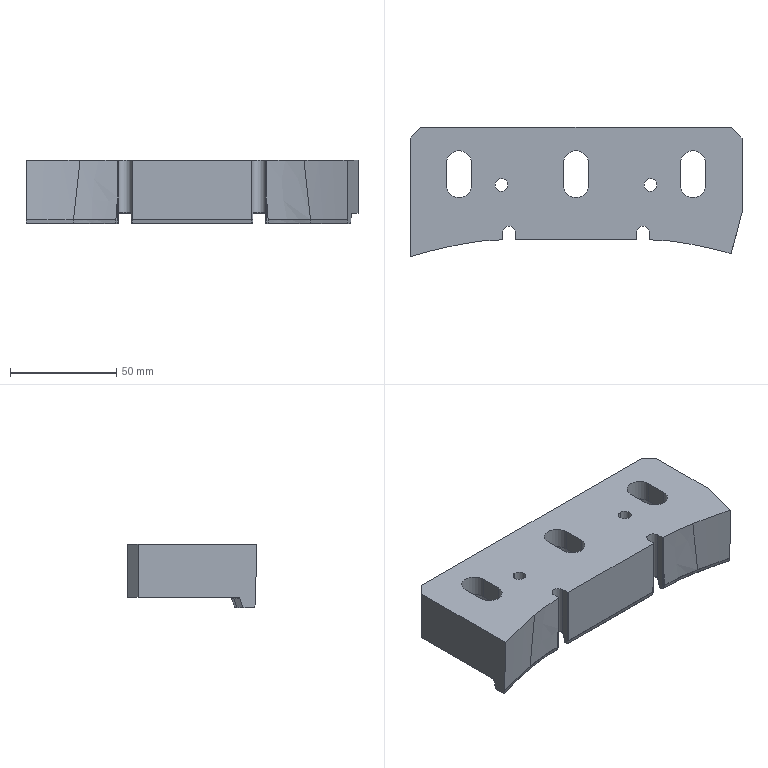CAM job | Mastercam | 3-axis milling | part box 156 x 60.706 x 30 mm
Tools:
tool_number,name,type,diameter_mm,corner_radius_mm,flutes,flute_length_mm,overall_length_mm,shoulder_length_mm,holder_diameter_mm,length_offset,diameter_offset,default_rpm,default_feed_mm_min,default_plunge_mm_min,coolant
1,63 Flat End Mill,end mill,63,0,4,25,75,25,50,1,1,159,19.08,600,COOL_OFF
2,6 Flat End Mill,end mill,6,0,4,25,75,25,50,2,2,1667,200.04,600,COOL_OFF
4,4 Flat End Mill,end mill,4,0,4,25,75,25,50,4,4,2500,300,600,COOL_OFF
6,6 Flat End Mill,end mill,6,0,4,25,75,25,50,6,6,1667,200.04,600,COOL_OFF
10,10 Flat End Mill,end mill,10,0,4,25,75,25,50,10,10,1000,120,600,COOL_OFF
11,10 Flat End Mill,end mill,10,0,4,25,75,25,50,11,11,1000,120,600,COOL_OFF
14,4 Flat End Mill,end mill,4,0,4,25,75,25,50,14,14,2500,300,600,COOL_OFF
16,16 Flat End Mill,end mill,16,0,4,25,100,25,50,16,16,750,90,600,COOL_OFF
17,12 Bull Nose Mill,bull end mill,12,0.5,4,12,24,14.4,50,17,17,2000,3000,600,COOL_FLOOD
17,12 Bull Nose Mill,bull end mill,12,0.5,4,12,24,14.4,50,17,17,2000,3000,600,COOL_FLOOD
18,6 Bull Nose Mill,bull end mill,6,0.5,4,25,100,25,50,18,18,2000,240,600,COOL_OFF
20,20 Bull Nose Mill,bull end mill,20,0.8,4,25,100,25,50,20,20,600,72,600,COOL_OFF
21,6 Chamfer Mill,chamfer mill,6,0,4,25,75,30,50,21,21,4166,499.92,600,COOL_OFF
Operations:
seq,operation,operation_type,tool_number,tool_name,tool_diameter_mm,spindle_rpm,feed_mm_min,plunge_mm_min,retract_mm_min,cycle_time_s,wcs,posted,nc_file
1,Contour (2D) - [WCS: Top] - [Tplane: Top],Contour,1,63 Flat End Mill,63,800,300,600,1200,109.406,Top,yes,.nc
2,Contour (Ramp) - [WCS: Top] - [Tplane: Top],Contour,20,20 Bull Nose Mill,20,1800,3000,600,1200,1027.969,Top,yes,.nc
3,Contour (Ramp) - [WCS: Top] - [Tplane: Top],Contour,10,10 Flat End Mill,10,1600,1400,600,1200,175.98,Top,yes,.nc
4,Contour (2D) - [WCS: Top] - [Tplane: Top],Contour,11,10 Flat End Mill,10,1800,500,600,1200,119.901,Top,yes,.nc
5,Contour (2D) - [WCS: Top] - [Tplane: Top],Contour,11,10 Flat End Mill,10,1600,400,600,1200,21.799,Top,yes,.nc
6,Contour (Ramp) - [WCS: Top] - [Tplane: Top],Contour,4,4 Flat End Mill,4,1600,1400,600,1200,292.647,Top,yes,.nc
7,Contour (2D) - [WCS: Top] - [Tplane: Top],Contour,14,4 Flat End Mill,4,1600,300,600,1200,29.003,Top,yes,.nc
8,Contour (Ramp) - [WCS: Top] - [Tplane: Top],Contour,4,4 Flat End Mill,4,2500,1400,600,1200,32.533,Top,yes,.nc
9,Contour (2D) - [WCS: Top] - [Tplane: Top],Contour,14,4 Flat End Mill,4,1600,300,600,1200,18.414,Top,yes,.nc
10,Contour (2D) - [WCS: Top] - [Tplane: Top],Contour,14,4 Flat End Mill,4,1600,300,600,1200,18.43,Top,yes,.nc
11,Contour (2D chamfer) - [WCS: Top] - [Tplane: Top],Contour,21,6 Chamfer Mill,6,2000,500,600,1200,86.852,Top,yes,.nc
12,Facing - [WCS: Top] - [Tplane: Top],Facing,20,20 Bull Nose Mill,20,1800,3000,600,1200,810.447,Top,yes,.nc
13,Facing - [WCS: Top] - [Tplane: Top],Facing,20,20 Bull Nose Mill,20,1800,500,600,1200,155.561,Top,yes,.nc
14,Contour (Ramp) - [WCS: Top] - [Tplane: Top],Contour,20,20 Bull Nose Mill,20,1800,3000,600,1200,212.462,Top,yes,.nc
15,Surface Finish Parallel - [WCS: Top] - [Tplane: Top],MultiSurfaceFinishParallel,18,6 Bull Nose Mill,6,1800,3000,600,1200,29.078,Top,yes,.nc
16,Surface Finish Contour - [WCS: Top] - [Tplane: Top],MultiSurfaceFinishContour,18,6 Bull Nose Mill,6,1800,3000,600,1200,46.827,Top,yes,.nc
17,Surface Finish Contour - [WCS: Top] - [Tplane: Top],MultiSurfaceFinishContour,18,6 Bull Nose Mill,6,1800,3000,600,1200,50.142,Top,yes,.nc
18,Contour (2D) - [WCS: Top] - [Tplane: Top],Contour,18,6 Bull Nose Mill,6,2000,800,600,1200,221.975,Top,yes,.nc
19,Contour (Ramp) - [WCS: Top] - [Tplane: Top],Contour,16,16 Flat End Mill,16,1800,2000,600,1200,244.39,Top,yes,.nc
20,Contour (2D) - [WCS: Top] - [Tplane: Top],Contour,11,10 Flat End Mill,10,1800,400,600,1200,38.044,Top,yes,.nc
21,Surface Finish Parallel - [WCS: Top] - [Tplane: Top],MultiSurfaceFinishParallel,18,6 Bull Nose Mill,6,1800,3000,600,1200,240.87,Top,yes,.nc
22,Surface Finish Contour - [WCS: Top] - [Tplane: Top],MultiSurfaceFinishContour,18,6 Bull Nose Mill,6,1800,3000,600,1200,133.271,Top,yes,.nc
23,Surface Finish Contour - [WCS: Top] - [Tplane: Top],MultiSurfaceFinishContour,18,6 Bull Nose Mill,6,1800,3000,600,1200,145.735,Top,yes,.nc
24,Contour (Ramp) - [WCS: Top] - [Tplane: Top],Contour,6,6 Flat End Mill,6,1600,1200,600,1200,48.063,Top,yes,.nc
25,Contour (2D) - [WCS: Top] - [Tplane: Top],Contour,2,6 Flat End Mill,6,1600,300,600,1200,13.64,Top,yes,.nc
26,Surface Finish Contour - [WCS: Top] - [Tplane: Top],MultiSurfaceFinishContour,18,6 Bull Nose Mill,6,2000,3000,600,1200,558.624,Top,yes,.nc
27,Surface Finish Contour - [WCS: Top] - [Tplane: Top],MultiSurfaceFinishContour,18,6 Bull Nose Mill,6,2000,3000,600,1200,664.856,Top,yes,.nc
28,Surface Finish Contour - [WCS: Top] - [Tplane: Top],MultiSurfaceFinishContour,18,6 Bull Nose Mill,6,2000,3000,600,1200,509.983,Top,yes,.nc
29,Contour (2D chamfer) - [WCS: Top] - [Tplane: Top],Contour,21,6 Chamfer Mill,6,2000,500,600,1200,47.734,Top,yes,.nc
30,Contour (2D chamfer) - [WCS: Top] - [Tplane: Top],Contour,21,6 Chamfer Mill,6,2000,500,600,1200,31.908,Top,yes,.nc